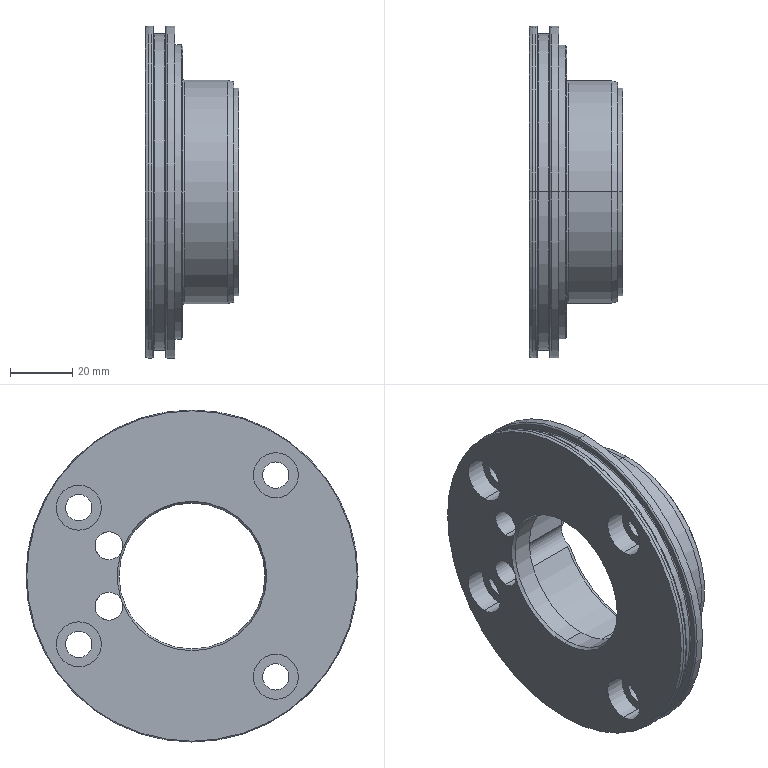Part | SolidWorks | features BaseBody 1 | 1 solid | 76 faces | box 30 x 107 x 107 mm | volume 84121 mm3 | cylinder 38 | torus 14 | cone 12 | plane 12 | commonest cylinder face diameters 8.5 x8 14.5 x8 9 x4 62 x4 107 x4 47 x2